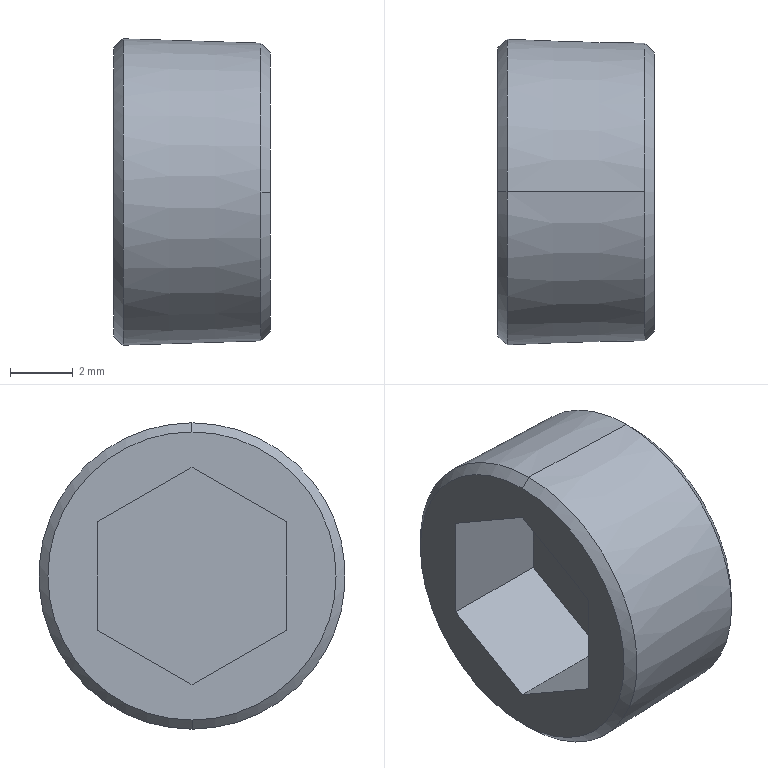Part | STEP file | 1 solid | 15 faces | box 5 x 9.772 x 9.772 mm | volume 252.752 mm3 | plane 9 | cone 6
STEP:
#1=CARTESIAN_POINT('',(0.,0.,0.));
#2=DIRECTION('',(0.,0.,1.));
#3=DIRECTION('',(1.,0.,0.));
#4=AXIS2_PLACEMENT_3D('',#1,#2,#3);
#5=CARTESIAN_POINT('',(5.,4.439,0.));
#6=VERTEX_POINT('',#5);
#7=CARTESIAN_POINT('',(5.,-4.439,0.));
#8=VERTEX_POINT('',#7);
#9=CARTESIAN_POINT('',(5.,0.,0.));
#10=DIRECTION('',(1.,0.,0.));
#11=DIRECTION('',(0.,-1.,0.));
#12=AXIS2_PLACEMENT_3D('',#9,#10,#11);
#13=CIRCLE('',#12,4.439);
#14=CARTESIAN_POINT('',(5.,0.,0.));
#15=DIRECTION('',(-1.,0.,0.));
#16=DIRECTION('',(0.,-1.,0.));
#17=AXIS2_PLACEMENT_3D('',#14,#15,#16);
#18=CONICAL_SURFACE('',#17,4.439,0.801);
#19=CARTESIAN_POINT('',(6.283,0.));
#20=DIRECTION('',(-1.,0.));
#21=VECTOR('',#20,1.);
#22=LINE('',#19,#21);
#23=(GEOMETRIC_REPRESENTATION_CONTEXT(2)PARAMETRIC_REPRESENTATION_CONTEXT()REPRESENTATION_CONTEXT('',''));
#24=DEFINITIONAL_REPRESENTATION('',(#22),#23);
#25=PCURVE('',#18,#24);
#26=CARTESIAN_POINT('',(5.,-4.492,-4.492));
#27=DIRECTION('',(-1.,0.,0.));
#28=DIRECTION('',(0.,0.,1.));
#29=AXIS2_PLACEMENT_3D('',#26,#27,#28);
#30=PLANE('',#29);
#31=CARTESIAN_POINT('',(4.492,0.05327));
#32=CARTESIAN_POINT('',(-3.196,0.05327));
#33=CARTESIAN_POINT('',(0.648,6.712));
#34=CARTESIAN_POINT('',(4.492,13.371));
#35=CARTESIAN_POINT('',(8.337,6.712));
#36=CARTESIAN_POINT('',(12.181,0.05327));
#37=CARTESIAN_POINT('',(4.492,0.05327));
#38=(BOUNDED_CURVE()B_SPLINE_CURVE(2,(#31,#32,#33,#34,#35,#36,#37),.UNSPECIFIED.,.T.,.F.)B_SPLINE_CURVE_WITH_KNOTS((1,2,2,2,2,1),(-2.094,0.,2.094,4.189,6.283,8.378),.UNSPECIFIED.)CURVE()GEOMETRIC_REPRESENTATION_ITEM()RATIONAL_B_SPLINE_CURVE((1.,0.5,1.,0.5,1.,0.5,1.))REPRESENTATION_ITEM(''));
#39=(GEOMETRIC_REPRESENTATION_CONTEXT(2)PARAMETRIC_REPRESENTATION_CONTEXT()REPRESENTATION_CONTEXT('',''));
#40=DEFINITIONAL_REPRESENTATION('',(#38),#39);
#41=PCURVE('',#30,#40);
#42=SURFACE_CURVE('',#13,(#25,#41),.PCURVE_S1.);
#43=EDGE_CURVE('',#6,#8,#42,.T.);
#44=ORIENTED_EDGE('',*,*,#43,.F.);
#45=CARTESIAN_POINT('',(4.7,4.748,0.));
#46=VERTEX_POINT('',#45);
#47=CARTESIAN_POINT('',(5.,4.439,0.));
#48=DIRECTION('',(-0.696,0.7181,0.));
#49=VECTOR('',#48,1.);
#50=LINE('',#47,#49);
#51=CARTESIAN_POINT('',(3.142,0.));
#52=DIRECTION('',(0.,1.));
#53=VECTOR('',#52,1.);
#54=LINE('',#51,#53);
#55=(GEOMETRIC_REPRESENTATION_CONTEXT(2)PARAMETRIC_REPRESENTATION_CONTEXT()REPRESENTATION_CONTEXT('',''));
#56=DEFINITIONAL_REPRESENTATION('',(#54),#55);
#57=PCURVE('',#18,#56);
#58=CARTESIAN_POINT('',(5.,0.,0.));
#59=DIRECTION('',(-1.,0.,0.));
#60=DIRECTION('',(0.,-1.,0.));
#61=AXIS2_PLACEMENT_3D('',#58,#59,#60);
#62=CONICAL_SURFACE('',#61,4.439,0.801);
#63=CARTESIAN_POINT('',(3.142,0.));
#64=DIRECTION('',(0.,1.));
#65=VECTOR('',#64,1.);
#66=LINE('',#63,#65);
#67=(GEOMETRIC_REPRESENTATION_CONTEXT(2)PARAMETRIC_REPRESENTATION_CONTEXT()REPRESENTATION_CONTEXT('',''));
#68=DEFINITIONAL_REPRESENTATION('',(#66),#67);
#69=PCURVE('',#62,#68);
#70=SURFACE_CURVE('',#50,(#57,#69),.PCURVE_S1.);
#71=EDGE_CURVE('',#6,#46,#70,.T.);
#72=ORIENTED_EDGE('',*,*,#71,.T.);
#73=CARTESIAN_POINT('',(4.7,0.,4.748));
#74=VERTEX_POINT('',#73);
#75=CARTESIAN_POINT('',(4.7,0.,0.));
#76=DIRECTION('',(-1.,0.,0.));
#77=DIRECTION('',(0.,0.,1.));
#78=AXIS2_PLACEMENT_3D('',#75,#76,#77);
#79=CIRCLE('',#78,4.748);
#80=CARTESIAN_POINT('',(1.571,0.2999));
#81=DIRECTION('',(1.,0.));
#82=VECTOR('',#81,1.);
#83=LINE('',#80,#82);
#84=(GEOMETRIC_REPRESENTATION_CONTEXT(2)PARAMETRIC_REPRESENTATION_CONTEXT()REPRESENTATION_CONTEXT('',''));
#85=DEFINITIONAL_REPRESENTATION('',(#83),#84);
#86=PCURVE('',#18,#85);
#87=CARTESIAN_POINT('',(4.7,0.,0.));
#88=DIRECTION('',(-1.,0.,0.));
#89=DIRECTION('',(0.,0.,1.));
#90=AXIS2_PLACEMENT_3D('',#87,#88,#89);
#91=CONICAL_SURFACE('',#90,4.748,0.03121);
#92=CARTESIAN_POINT('',(0.,0.));
#93=DIRECTION('',(1.,0.));
#94=VECTOR('',#93,1.);
#95=LINE('',#92,#94);
#96=(GEOMETRIC_REPRESENTATION_CONTEXT(2)PARAMETRIC_REPRESENTATION_CONTEXT()REPRESENTATION_CONTEXT('',''));
#97=DEFINITIONAL_REPRESENTATION('',(#95),#96);
#98=PCURVE('',#91,#97);
#99=SURFACE_CURVE('',#79,(#86,#98),.PCURVE_S1.);
#100=EDGE_CURVE('',#74,#46,#99,.T.);
#101=ORIENTED_EDGE('',*,*,#100,.F.);
#102=CARTESIAN_POINT('',(4.7,-4.748,0.));
#103=VERTEX_POINT('',#102);
#104=CARTESIAN_POINT('',(4.7,0.,0.));
#105=DIRECTION('',(-1.,0.,0.));
#106=DIRECTION('',(0.,0.,1.));
#107=AXIS2_PLACEMENT_3D('',#104,#105,#106);
#108=CIRCLE('',#107,4.748);
#109=CARTESIAN_POINT('',(-4.712,0.2999));
#110=DIRECTION('',(1.,0.));
#111=VECTOR('',#110,1.);
#112=LINE('',#109,#111);
#113=(GEOMETRIC_REPRESENTATION_CONTEXT(2)PARAMETRIC_REPRESENTATION_CONTEXT()REPRESENTATION_CONTEXT('',''));
#114=DEFINITIONAL_REPRESENTATION('',(#112),#113);
#115=PCURVE('',#18,#114);
#116=CARTESIAN_POINT('',(4.7,0.,0.));
#117=DIRECTION('',(-1.,0.,0.));
#118=DIRECTION('',(0.,0.,1.));
#119=AXIS2_PLACEMENT_3D('',#116,#117,#118);
#120=CONICAL_SURFACE('',#119,4.748,0.03121);
#121=CARTESIAN_POINT('',(0.,0.));
#122=DIRECTION('',(1.,0.));
#123=VECTOR('',#122,1.);
#124=LINE('',#121,#123);
#125=(GEOMETRIC_REPRESENTATION_CONTEXT(2)PARAMETRIC_REPRESENTATION_CONTEXT()REPRESENTATION_CONTEXT('',''));
#126=DEFINITIONAL_REPRESENTATION('',(#124),#125);
#127=PCURVE('',#120,#126);
#128=SURFACE_CURVE('',#108,(#115,#127),.PCURVE_S1.);
#129=EDGE_CURVE('',#103,#74,#128,.T.);
#130=ORIENTED_EDGE('',*,*,#129,.F.);
#131=CARTESIAN_POINT('',(5.,-4.439,0.));
#132=DIRECTION('',(-0.696,-0.7181,0.));
#133=VECTOR('',#132,1.);
#134=LINE('',#131,#133);
#135=CARTESIAN_POINT('',(0.,0.));
#136=DIRECTION('',(0.,1.));
#137=VECTOR('',#136,1.);
#138=LINE('',#135,#137);
#139=(GEOMETRIC_REPRESENTATION_CONTEXT(2)PARAMETRIC_REPRESENTATION_CONTEXT()REPRESENTATION_CONTEXT('',''));
#140=DEFINITIONAL_REPRESENTATION('',(#138),#139);
#141=PCURVE('',#18,#140);
#142=CARTESIAN_POINT('',(6.283,0.));
#143=DIRECTION('',(0.,1.));
#144=VECTOR('',#143,1.);
#145=LINE('',#142,#144);
#146=(GEOMETRIC_REPRESENTATION_CONTEXT(2)PARAMETRIC_REPRESENTATION_CONTEXT()REPRESENTATION_CONTEXT('',''));
#147=DEFINITIONAL_REPRESENTATION('',(#145),#146);
#148=PCURVE('',#62,#147);
#149=SURFACE_CURVE('',#134,(#141,#148),.PCURVE_S1.);
#150=EDGE_CURVE('',#8,#103,#149,.T.);
#151=ORIENTED_EDGE('',*,*,#150,.F.);
#152=EDGE_LOOP('',(#44,#72,#101,#130,#151));
#153=FACE_BOUND('',#152,.T.);
#154=ADVANCED_FACE('',(#153),#18,.T.);
#155=ORIENTED_EDGE('',*,*,#100,.T.);
#156=CARTESIAN_POINT('',(4.7,0.,-4.748));
#157=VERTEX_POINT('',#156);
#158=CARTESIAN_POINT('',(4.7,0.,0.));
#159=DIRECTION('',(-1.,0.,0.));
#160=DIRECTION('',(0.,0.,1.));
#161=AXIS2_PLACEMENT_3D('',#158,#159,#160);
#162=CIRCLE('',#161,4.748);
#163=CARTESIAN_POINT('',(0.,0.));
#164=DIRECTION('',(1.,0.));
#165=VECTOR('',#164,1.);
#166=LINE('',#163,#165);
#167=(GEOMETRIC_REPRESENTATION_CONTEXT(2)PARAMETRIC_REPRESENTATION_CONTEXT()REPRESENTATION_CONTEXT('',''));
#168=DEFINITIONAL_REPRESENTATION('',(#166),#167);
#169=PCURVE('',#91,#168);
#170=CARTESIAN_POINT('',(1.571,0.2999));
#171=DIRECTION('',(1.,0.));
#172=VECTOR('',#171,1.);
#173=LINE('',#170,#172);
#174=(GEOMETRIC_REPRESENTATION_CONTEXT(2)PARAMETRIC_REPRESENTATION_CONTEXT()REPRESENTATION_CONTEXT('',''));
#175=DEFINITIONAL_REPRESENTATION('',(#173),#174);
#176=PCURVE('',#62,#175);
#177=SURFACE_CURVE('',#162,(#169,#176),.PCURVE_S1.);
#178=EDGE_CURVE('',#46,#157,#177,.T.);
#179=ORIENTED_EDGE('',*,*,#178,.T.);
#180=CARTESIAN_POINT('',(0.2999,0.,-4.886));
#181=VERTEX_POINT('',#180);
#182=CARTESIAN_POINT('',(4.7,0.,-4.748));
#183=DIRECTION('',(-0.9995,0.,-0.0312));
#184=VECTOR('',#183,1.);
#185=LINE('',#182,#184);
#186=CARTESIAN_POINT('',(3.142,0.));
#187=DIRECTION('',(0.,1.));
#188=VECTOR('',#187,1.);
#189=LINE('',#186,#188);
#190=(GEOMETRIC_REPRESENTATION_CONTEXT(2)PARAMETRIC_REPRESENTATION_CONTEXT()REPRESENTATION_CONTEXT('',''));
#191=DEFINITIONAL_REPRESENTATION('',(#189),#190);
#192=PCURVE('',#91,#191);
#193=CARTESIAN_POINT('',(3.142,0.));
#194=DIRECTION('',(0.,1.));
#195=VECTOR('',#194,1.);
#196=LINE('',#193,#195);
#197=(GEOMETRIC_REPRESENTATION_CONTEXT(2)PARAMETRIC_REPRESENTATION_CONTEXT()REPRESENTATION_CONTEXT('',''));
#198=DEFINITIONAL_REPRESENTATION('',(#196),#197);
#199=PCURVE('',#120,#198);
#200=SURFACE_CURVE('',#185,(#192,#199),.PCURVE_S1.);
#201=EDGE_CURVE('',#157,#181,#200,.T.);
#202=ORIENTED_EDGE('',*,*,#201,.T.);
#203=CARTESIAN_POINT('',(0.2999,0.,4.886));
#204=VERTEX_POINT('',#203);
#205=CARTESIAN_POINT('',(0.2999,0.,0.));
#206=DIRECTION('',(-1.,0.,0.));
#207=DIRECTION('',(0.,0.,1.));
#208=AXIS2_PLACEMENT_3D('',#205,#206,#207);
#209=CIRCLE('',#208,4.886);
#210=CARTESIAN_POINT('',(0.,4.4));
#211=DIRECTION('',(1.,0.));
#212=VECTOR('',#211,1.);
#213=LINE('',#210,#212);
#214=(GEOMETRIC_REPRESENTATION_CONTEXT(2)PARAMETRIC_REPRESENTATION_CONTEXT()REPRESENTATION_CONTEXT('',''));
#215=DEFINITIONAL_REPRESENTATION('',(#213),#214);
#216=PCURVE('',#91,#215);
#217=CARTESIAN_POINT('',(0.,0.,0.));
#218=DIRECTION('',(1.,0.,0.));
#219=DIRECTION('',(0.,0.,-1.));
#220=AXIS2_PLACEMENT_3D('',#217,#218,#219);
#221=CONICAL_SURFACE('',#220,4.595,0.7698);
#222=CARTESIAN_POINT('',(3.142,0.2999));
#223=DIRECTION('',(-1.,0.));
#224=VECTOR('',#223,1.);
#225=LINE('',#222,#224);
#226=(GEOMETRIC_REPRESENTATION_CONTEXT(2)PARAMETRIC_REPRESENTATION_CONTEXT()REPRESENTATION_CONTEXT('',''));
#227=DEFINITIONAL_REPRESENTATION('',(#225),#226);
#228=PCURVE('',#221,#227);
#229=SURFACE_CURVE('',#209,(#216,#228),.PCURVE_S1.);
#230=EDGE_CURVE('',#204,#181,#229,.T.);
#231=ORIENTED_EDGE('',*,*,#230,.F.);
#232=CARTESIAN_POINT('',(4.7,0.,4.748));
#233=DIRECTION('',(-0.9995,0.,0.0312));
#234=VECTOR('',#233,1.);
#235=LINE('',#232,#234);
#236=CARTESIAN_POINT('',(0.,0.));
#237=DIRECTION('',(0.,1.));
#238=VECTOR('',#237,1.);
#239=LINE('',#236,#238);
#240=(GEOMETRIC_REPRESENTATION_CONTEXT(2)PARAMETRIC_REPRESENTATION_CONTEXT()REPRESENTATION_CONTEXT('',''));
#241=DEFINITIONAL_REPRESENTATION('',(#239),#240);
#242=PCURVE('',#91,#241);
#243=CARTESIAN_POINT('',(6.283,0.));
#244=DIRECTION('',(0.,1.));
#245=VECTOR('',#244,1.);
#246=LINE('',#243,#245);
#247=(GEOMETRIC_REPRESENTATION_CONTEXT(2)PARAMETRIC_REPRESENTATION_CONTEXT()REPRESENTATION_CONTEXT('',''));
#248=DEFINITIONAL_REPRESENTATION('',(#246),#247);
#249=PCURVE('',#120,#248);
#250=SURFACE_CURVE('',#235,(#242,#249),.PCURVE_S1.);
#251=EDGE_CURVE('',#74,#204,#250,.T.);
#252=ORIENTED_EDGE('',*,*,#251,.F.);
#253=EDGE_LOOP('',(#155,#179,#202,#231,#252));
#254=FACE_BOUND('',#253,.T.);
#255=ADVANCED_FACE('',(#254),#91,.T.);
#256=CARTESIAN_POINT('',(0.,0.,4.595));
#257=VERTEX_POINT('',#256);
#258=CARTESIAN_POINT('',(0.,0.,-4.595));
#259=VERTEX_POINT('',#258);
#260=CARTESIAN_POINT('',(0.,0.,0.));
#261=DIRECTION('',(-1.,0.,0.));
#262=DIRECTION('',(0.,0.,-1.));
#263=AXIS2_PLACEMENT_3D('',#260,#261,#262);
#264=CIRCLE('',#263,4.595);
#265=CARTESIAN_POINT('',(6.283,0.));
#266=DIRECTION('',(-1.,0.));
#267=VECTOR('',#266,1.);
#268=LINE('',#265,#267);
#269=(GEOMETRIC_REPRESENTATION_CONTEXT(2)PARAMETRIC_REPRESENTATION_CONTEXT()REPRESENTATION_CONTEXT('',''));
#270=DEFINITIONAL_REPRESENTATION('',(#268),#269);
#271=PCURVE('',#221,#270);
#272=CARTESIAN_POINT('',(0.,-4.65,4.65));
#273=DIRECTION('',(1.,0.,0.));
#274=DIRECTION('',(0.,0.,-1.));
#275=AXIS2_PLACEMENT_3D('',#272,#273,#274);
#276=PLANE('',#275);
#277=CARTESIAN_POINT('',(9.246,4.65));
#278=CARTESIAN_POINT('',(9.246,-3.309));
#279=CARTESIAN_POINT('',(2.353,0.6708));
#280=CARTESIAN_POINT('',(-4.54,4.65));
#281=CARTESIAN_POINT('',(2.353,8.63));
#282=CARTESIAN_POINT('',(9.246,12.61));
#283=CARTESIAN_POINT('',(9.246,4.65));
#284=(BOUNDED_CURVE()B_SPLINE_CURVE(2,(#277,#278,#279,#280,#281,#282,#283),.UNSPECIFIED.,.T.,.F.)B_SPLINE_CURVE_WITH_KNOTS((1,2,2,2,2,1),(-2.094,0.,2.094,4.189,6.283,8.378),.UNSPECIFIED.)CURVE()GEOMETRIC_REPRESENTATION_ITEM()RATIONAL_B_SPLINE_CURVE((1.,0.5,1.,0.5,1.,0.5,1.))REPRESENTATION_ITEM(''));
#285=(GEOMETRIC_REPRESENTATION_CONTEXT(2)PARAMETRIC_REPRESENTATION_CONTEXT()REPRESENTATION_CONTEXT('',''));
#286=DEFINITIONAL_REPRESENTATION('',(#284),#285);
#287=PCURVE('',#276,#286);
#288=SURFACE_CURVE('',#264,(#271,#287),.PCURVE_S1.);
#289=EDGE_CURVE('',#257,#259,#288,.T.);
#290=ORIENTED_EDGE('',*,*,#289,.F.);
#291=CARTESIAN_POINT('',(0.,0.,4.595));
#292=DIRECTION('',(0.7181,0.,0.696));
#293=VECTOR('',#292,1.);
#294=LINE('',#291,#293);
#295=CARTESIAN_POINT('',(3.142,0.));
#296=DIRECTION('',(0.,1.));
#297=VECTOR('',#296,1.);
#298=LINE('',#295,#297);
#299=(GEOMETRIC_REPRESENTATION_CONTEXT(2)PARAMETRIC_REPRESENTATION_CONTEXT()REPRESENTATION_CONTEXT('',''));
#300=DEFINITIONAL_REPRESENTATION('',(#298),#299);
#301=PCURVE('',#221,#300);
#302=CARTESIAN_POINT('',(0.,0.,0.));
#303=DIRECTION('',(1.,0.,0.));
#304=DIRECTION('',(0.,0.,-1.));
#305=AXIS2_PLACEMENT_3D('',#302,#303,#304);
#306=CONICAL_SURFACE('',#305,4.595,0.7698);
#307=CARTESIAN_POINT('',(3.142,0.));
#308=DIRECTION('',(0.,1.));
#309=VECTOR('',#308,1.);
#310=LINE('',#307,#309);
#311=(GEOMETRIC_REPRESENTATION_CONTEXT(2)PARAMETRIC_REPRESENTATION_CONTEXT()REPRESENTATION_CONTEXT('',''));
#312=DEFINITIONAL_REPRESENTATION('',(#310),#311);
#313=PCURVE('',#306,#312);
#314=SURFACE_CURVE('',#294,(#301,#313),.PCURVE_S1.);
#315=EDGE_CURVE('',#257,#204,#314,.T.);
#316=ORIENTED_EDGE('',*,*,#315,.T.);
#317=ORIENTED_EDGE('',*,*,#230,.T.);
#318=CARTESIAN_POINT('',(0.,0.,-4.595));
#319=DIRECTION('',(0.7181,0.,-0.696));
#320=VECTOR('',#319,1.);
#321=LINE('',#318,#320);
#322=CARTESIAN_POINT('',(0.,0.));
#323=DIRECTION('',(0.,1.));
#324=VECTOR('',#323,1.);
#325=LINE('',#322,#324);
#326=(GEOMETRIC_REPRESENTATION_CONTEXT(2)PARAMETRIC_REPRESENTATION_CONTEXT()REPRESENTATION_CONTEXT('',''));
#327=DEFINITIONAL_REPRESENTATION('',(#325),#326);
#328=PCURVE('',#221,#327);
#329=CARTESIAN_POINT('',(6.283,0.));
#330=DIRECTION('',(0.,1.));
#331=VECTOR('',#330,1.);
#332=LINE('',#329,#331);
#333=(GEOMETRIC_REPRESENTATION_CONTEXT(2)PARAMETRIC_REPRESENTATION_CONTEXT()REPRESENTATION_CONTEXT('',''));
#334=DEFINITIONAL_REPRESENTATION('',(#332),#333);
#335=PCURVE('',#306,#334);
#336=SURFACE_CURVE('',#321,(#328,#335),.PCURVE_S1.);
#337=EDGE_CURVE('',#259,#181,#336,.T.);
#338=ORIENTED_EDGE('',*,*,#337,.F.);
#339=EDGE_LOOP('',(#290,#316,#317,#338));
#340=FACE_BOUND('',#339,.T.);
#341=ADVANCED_FACE('',(#340),#221,.T.);
#342=ORIENTED_EDGE('',*,*,#71,.F.);
#343=CARTESIAN_POINT('',(5.,0.,0.));
#344=DIRECTION('',(1.,0.,0.));
#345=DIRECTION('',(0.,-1.,0.));
#346=AXIS2_PLACEMENT_3D('',#343,#344,#345);
#347=CIRCLE('',#346,4.439);
#348=CARTESIAN_POINT('',(6.283,0.));
#349=DIRECTION('',(-1.,0.));
#350=VECTOR('',#349,1.);
#351=LINE('',#348,#350);
#352=(GEOMETRIC_REPRESENTATION_CONTEXT(2)PARAMETRIC_REPRESENTATION_CONTEXT()REPRESENTATION_CONTEXT('',''));
#353=DEFINITIONAL_REPRESENTATION('',(#351),#352);
#354=PCURVE('',#62,#353);
#355=CARTESIAN_POINT('',(4.492,0.05327));
#356=CARTESIAN_POINT('',(-3.196,0.05327));
#357=CARTESIAN_POINT('',(0.648,6.712));
#358=CARTESIAN_POINT('',(4.492,13.371));
#359=CARTESIAN_POINT('',(8.337,6.712));
#360=CARTESIAN_POINT('',(12.181,0.05327));
#361=CARTESIAN_POINT('',(4.492,0.05327));
#362=(BOUNDED_CURVE()B_SPLINE_CURVE(2,(#355,#356,#357,#358,#359,#360,#361),.UNSPECIFIED.,.T.,.F.)B_SPLINE_CURVE_WITH_KNOTS((1,2,2,2,2,1),(-2.094,0.,2.094,4.189,6.283,8.378),.UNSPECIFIED.)CURVE()GEOMETRIC_REPRESENTATION_ITEM()RATIONAL_B_SPLINE_CURVE((1.,0.5,1.,0.5,1.,0.5,1.))REPRESENTATION_ITEM(''));
#363=(GEOMETRIC_REPRESENTATION_CONTEXT(2)PARAMETRIC_REPRESENTATION_CONTEXT()REPRESENTATION_CONTEXT('',''));
#364=DEFINITIONAL_REPRESENTATION('',(#362),#363);
#365=PCURVE('',#30,#364);
#366=SURFACE_CURVE('',#347,(#354,#365),.PCURVE_S1.);
#367=EDGE_CURVE('',#8,#6,#366,.T.);
#368=ORIENTED_EDGE('',*,*,#367,.F.);
#369=ORIENTED_EDGE('',*,*,#150,.T.);
#370=CARTESIAN_POINT('',(4.7,0.,0.));
#371=DIRECTION('',(-1.,0.,0.));
#372=DIRECTION('',(0.,0.,1.));
#373=AXIS2_PLACEMENT_3D('',#370,#371,#372);
#374=CIRCLE('',#373,4.748);
#375=CARTESIAN_POINT('',(1.571,0.2999));
#376=DIRECTION('',(1.,0.));
#377=VECTOR('',#376,1.);
#378=LINE('',#375,#377);
#379=(GEOMETRIC_REPRESENTATION_CONTEXT(2)PARAMETRIC_REPRESENTATION_CONTEXT()REPRESENTATION_CONTEXT('',''));
#380=DEFINITIONAL_REPRESENTATION('',(#378),#379);
#381=PCURVE('',#62,#380);
#382=CARTESIAN_POINT('',(0.,0.));
#383=DIRECTION('',(1.,0.));
#384=VECTOR('',#383,1.);
#385=LINE('',#382,#384);
#386=(GEOMETRIC_REPRESENTATION_CONTEXT(2)PARAMETRIC_REPRESENTATION_CONTEXT()REPRESENTATION_CONTEXT('',''));
#387=DEFINITIONAL_REPRESENTATION('',(#385),#386);
#388=PCURVE('',#120,#387);
#389=SURFACE_CURVE('',#374,(#381,#388),.PCURVE_S1.);
#390=EDGE_CURVE('',#157,#103,#389,.T.);
#391=ORIENTED_EDGE('',*,*,#390,.F.);
#392=ORIENTED_EDGE('',*,*,#178,.F.);
#393=EDGE_LOOP('',(#342,#368,#369,#391,#392));
#394=FACE_BOUND('',#393,.T.);
#395=ADVANCED_FACE('',(#394),#62,.T.);
#396=ORIENTED_EDGE('',*,*,#367,.T.);
#397=ORIENTED_EDGE('',*,*,#43,.T.);
#398=EDGE_LOOP('',(#396,#397));
#399=FACE_BOUND('',#398,.T.);
#400=ADVANCED_FACE('',(#399),#30,.F.);
#401=ORIENTED_EDGE('',*,*,#201,.F.);
#402=ORIENTED_EDGE('',*,*,#390,.T.);
#403=ORIENTED_EDGE('',*,*,#129,.T.);
#404=ORIENTED_EDGE('',*,*,#251,.T.);
#405=CARTESIAN_POINT('',(0.2999,0.,0.));
#406=DIRECTION('',(-1.,0.,0.));
#407=DIRECTION('',(0.,0.,1.));
#408=AXIS2_PLACEMENT_3D('',#405,#406,#407);
#409=CIRCLE('',#408,4.886);
#410=CARTESIAN_POINT('',(0.,4.4));
#411=DIRECTION('',(1.,0.));
#412=VECTOR('',#411,1.);
#413=LINE('',#410,#412);
#414=(GEOMETRIC_REPRESENTATION_CONTEXT(2)PARAMETRIC_REPRESENTATION_CONTEXT()REPRESENTATION_CONTEXT('',''));
#415=DEFINITIONAL_REPRESENTATION('',(#413),#414);
#416=PCURVE('',#120,#415);
#417=CARTESIAN_POINT('',(9.425,0.2999));
#418=DIRECTION('',(-1.,0.));
#419=VECTOR('',#418,1.);
#420=LINE('',#417,#419);
#421=(GEOMETRIC_REPRESENTATION_CONTEXT(2)PARAMETRIC_REPRESENTATION_CONTEXT()REPRESENTATION_CONTEXT('',''));
#422=DEFINITIONAL_REPRESENTATION('',(#420),#421);
#423=PCURVE('',#306,#422);
#424=SURFACE_CURVE('',#409,(#416,#423),.PCURVE_S1.);
#425=EDGE_CURVE('',#181,#204,#424,.T.);
#426=ORIENTED_EDGE('',*,*,#425,.F.);
#427=EDGE_LOOP('',(#401,#402,#403,#404,#426));
#428=FACE_BOUND('',#427,.T.);
#429=ADVANCED_FACE('',(#428),#120,.T.);
#430=ORIENTED_EDGE('',*,*,#315,.F.);
#431=CARTESIAN_POINT('',(0.,0.,0.));
#432=DIRECTION('',(-1.,0.,0.));
#433=DIRECTION('',(0.,0.,-1.));
#434=AXIS2_PLACEMENT_3D('',#431,#432,#433);
#435=CIRCLE('',#434,4.595);
#436=CARTESIAN_POINT('',(6.283,0.));
#437=DIRECTION('',(-1.,0.));
#438=VECTOR('',#437,1.);
#439=LINE('',#436,#438);
#440=(GEOMETRIC_REPRESENTATION_CONTEXT(2)PARAMETRIC_REPRESENTATION_CONTEXT()REPRESENTATION_CONTEXT('',''));
#441=DEFINITIONAL_REPRESENTATION('',(#439),#440);
#442=PCURVE('',#306,#441);
#443=CARTESIAN_POINT('',(9.246,4.65));
#444=CARTESIAN_POINT('',(9.246,-3.309));
#445=CARTESIAN_POINT('',(2.353,0.6708));
#446=CARTESIAN_POINT('',(-4.54,4.65));
#447=CARTESIAN_POINT('',(2.353,8.63));
#448=CARTESIAN_POINT('',(9.246,12.61));
#449=CARTESIAN_POINT('',(9.246,4.65));
#450=(BOUNDED_CURVE()B_SPLINE_CURVE(2,(#443,#444,#445,#446,#447,#448,#449),.UNSPECIFIED.,.T.,.F.)B_SPLINE_CURVE_WITH_KNOTS((1,2,2,2,2,1),(-2.094,0.,2.094,4.189,6.283,8.378),.UNSPECIFIED.)CURVE()GEOMETRIC_REPRESENTATION_ITEM()RATIONAL_B_SPLINE_CURVE((1.,0.5,1.,0.5,1.,0.5,1.))REPRESENTATION_ITEM(''));
#451=(GEOMETRIC_REPRESENTATION_CONTEXT(2)PARAMETRIC_REPRESENTATION_CONTEXT()REPRESENTATION_CONTEXT('',''));
#452=DEFINITIONAL_REPRESENTATION('',(#450),#451);
#453=PCURVE('',#276,#452);
#454=SURFACE_CURVE('',#435,(#442,#453),.PCURVE_S1.);
#455=EDGE_CURVE('',#259,#257,#454,.T.);
#456=ORIENTED_EDGE('',*,*,#455,.F.);
#457=ORIENTED_EDGE('',*,*,#337,.T.);
#458=ORIENTED_EDGE('',*,*,#425,.T.);
#459=EDGE_LOOP('',(#430,#456,#457,#458));
#460=FACE_BOUND('',#459,.T.);
#461=ADVANCED_FACE('',(#460),#306,.T.);
#462=CARTESIAN_POINT('',(0.,0.,-3.464));
#463=VERTEX_POINT('',#462);
#464=CARTESIAN_POINT('',(0.,-3.,-1.732));
#465=VERTEX_POINT('',#464);
#466=CARTESIAN_POINT('',(0.,-3.,-1.732));
#467=DIRECTION('',(0.,-0.866,0.5));
#468=VECTOR('',#467,1.);
#469=LINE('',#466,#468);
#470=CARTESIAN_POINT('',(6.382,1.65));
#471=DIRECTION('',(-0.5,-0.866));
#472=VECTOR('',#471,1.);
#473=LINE('',#470,#472);
#474=(GEOMETRIC_REPRESENTATION_CONTEXT(2)PARAMETRIC_REPRESENTATION_CONTEXT()REPRESENTATION_CONTEXT('',''));
#475=DEFINITIONAL_REPRESENTATION('',(#473),#474);
#476=PCURVE('',#276,#475);
#477=CARTESIAN_POINT('',(0.,-3.,-1.732));
#478=DIRECTION('',(0.,-0.5,-0.866));
#479=DIRECTION('',(0.,0.866,-0.5));
#480=AXIS2_PLACEMENT_3D('',#477,#478,#479);
#481=PLANE('',#480);
#482=CARTESIAN_POINT('',(0.,0.));
#483=DIRECTION('',(-1.,0.));
#484=VECTOR('',#483,1.);
#485=LINE('',#482,#484);
#486=(GEOMETRIC_REPRESENTATION_CONTEXT(2)PARAMETRIC_REPRESENTATION_CONTEXT()REPRESENTATION_CONTEXT('',''));
#487=DEFINITIONAL_REPRESENTATION('',(#485),#486);
#488=PCURVE('',#481,#487);
#489=SURFACE_CURVE('',#469,(#476,#488),.PCURVE_S1.);
#490=EDGE_CURVE('',#463,#465,#489,.T.);
#491=ORIENTED_EDGE('',*,*,#490,.F.);
#492=CARTESIAN_POINT('',(0.,3.,-1.732));
#493=VERTEX_POINT('',#492);
#494=CARTESIAN_POINT('',(0.,0.,-3.464));
#495=DIRECTION('',(0.,-0.866,-0.5));
#496=VECTOR('',#495,1.);
#497=LINE('',#494,#496);
#498=CARTESIAN_POINT('',(8.114,4.65));
#499=DIRECTION('',(0.5,-0.866));
#500=VECTOR('',#499,1.);
#501=LINE('',#498,#500);
#502=(GEOMETRIC_REPRESENTATION_CONTEXT(2)PARAMETRIC_REPRESENTATION_CONTEXT()REPRESENTATION_CONTEXT('',''));
#503=DEFINITIONAL_REPRESENTATION('',(#501),#502);
#504=PCURVE('',#276,#503);
#505=CARTESIAN_POINT('',(0.,0.,-3.464));
#506=DIRECTION('',(0.,0.5,-0.866));
#507=DIRECTION('',(0.,0.866,0.5));
#508=AXIS2_PLACEMENT_3D('',#505,#506,#507);
#509=PLANE('',#508);
#510=CARTESIAN_POINT('',(0.,0.));
#511=DIRECTION('',(-1.,0.));
#512=VECTOR('',#511,1.);
#513=LINE('',#510,#512);
#514=(GEOMETRIC_REPRESENTATION_CONTEXT(2)PARAMETRIC_REPRESENTATION_CONTEXT()REPRESENTATION_CONTEXT('',''));
#515=DEFINITIONAL_REPRESENTATION('',(#513),#514);
#516=PCURVE('',#509,#515);
#517=SURFACE_CURVE('',#497,(#504,#516),.PCURVE_S1.);
#518=EDGE_CURVE('',#493,#463,#517,.T.);
#519=ORIENTED_EDGE('',*,*,#518,.F.);
#520=CARTESIAN_POINT('',(0.,3.,1.732));
#521=VERTEX_POINT('',#520);
#522=CARTESIAN_POINT('',(0.,3.,0.));
#523=DIRECTION('',(0.,0.,-1.));
#524=VECTOR('',#523,1.);
#525=LINE('',#522,#524);
#526=CARTESIAN_POINT('',(4.65,7.65));
#527=DIRECTION('',(1.,0.));
#528=VECTOR('',#527,1.);
#529=LINE('',#526,#528);
#530=(GEOMETRIC_REPRESENTATION_CONTEXT(2)PARAMETRIC_REPRESENTATION_CONTEXT()REPRESENTATION_CONTEXT('',''));
#531=DEFINITIONAL_REPRESENTATION('',(#529),#530);
#532=PCURVE('',#276,#531);
#533=CARTESIAN_POINT('',(0.,3.,-1.732));
#534=DIRECTION('',(0.,1.,0.));
#535=DIRECTION('',(0.,0.,1.));
#536=AXIS2_PLACEMENT_3D('',#533,#534,#535);
#537=PLANE('',#536);
#538=CARTESIAN_POINT('',(1.732,0.));
#539=DIRECTION('',(-1.,0.));
#540=VECTOR('',#539,1.);
#541=LINE('',#538,#540);
#542=(GEOMETRIC_REPRESENTATION_CONTEXT(2)PARAMETRIC_REPRESENTATION_CONTEXT()REPRESENTATION_CONTEXT('',''));
#543=DEFINITIONAL_REPRESENTATION('',(#541),#542);
#544=PCURVE('',#537,#543);
#545=SURFACE_CURVE('',#525,(#532,#544),.PCURVE_S1.);
#546=EDGE_CURVE('',#521,#493,#545,.T.);
#547=ORIENTED_EDGE('',*,*,#546,.F.);
#548=CARTESIAN_POINT('',(0.,0.,3.464));
#549=VERTEX_POINT('',#548);
#550=CARTESIAN_POINT('',(0.,3.,1.732));
#551=DIRECTION('',(0.,0.866,-0.5));
#552=VECTOR('',#551,1.);
#553=LINE('',#550,#552);
#554=CARTESIAN_POINT('',(2.918,7.65));
#555=DIRECTION('',(0.5,0.866));
#556=VECTOR('',#555,1.);
#557=LINE('',#554,#556);
#558=(GEOMETRIC_REPRESENTATION_CONTEXT(2)PARAMETRIC_REPRESENTATION_CONTEXT()REPRESENTATION_CONTEXT('',''));
#559=DEFINITIONAL_REPRESENTATION('',(#557),#558);
#560=PCURVE('',#276,#559);
#561=CARTESIAN_POINT('',(0.,3.,1.732));
#562=DIRECTION('',(0.,0.5,0.866));
#563=DIRECTION('',(0.,-0.866,0.5));
#564=AXIS2_PLACEMENT_3D('',#561,#562,#563);
#565=PLANE('',#564);
#566=CARTESIAN_POINT('',(0.,0.));
#567=DIRECTION('',(-1.,0.));
#568=VECTOR('',#567,1.);
#569=LINE('',#566,#568);
#570=(GEOMETRIC_REPRESENTATION_CONTEXT(2)PARAMETRIC_REPRESENTATION_CONTEXT()REPRESENTATION_CONTEXT('',''));
#571=DEFINITIONAL_REPRESENTATION('',(#569),#570);
#572=PCURVE('',#565,#571);
#573=SURFACE_CURVE('',#553,(#560,#572),.PCURVE_S1.);
#574=EDGE_CURVE('',#549,#521,#573,.T.);
#575=ORIENTED_EDGE('',*,*,#574,.F.);
#576=CARTESIAN_POINT('',(0.,-3.,1.732));
#577=VERTEX_POINT('',#576);
#578=CARTESIAN_POINT('',(0.,0.,3.464));
#579=DIRECTION('',(0.,0.866,0.5));
#580=VECTOR('',#579,1.);
#581=LINE('',#578,#580);
#582=CARTESIAN_POINT('',(1.186,4.65));
#583=DIRECTION('',(-0.5,0.866));
#584=VECTOR('',#583,1.);
#585=LINE('',#582,#584);
#586=(GEOMETRIC_REPRESENTATION_CONTEXT(2)PARAMETRIC_REPRESENTATION_CONTEXT()REPRESENTATION_CONTEXT('',''));
#587=DEFINITIONAL_REPRESENTATION('',(#585),#586);
#588=PCURVE('',#276,#587);
#589=CARTESIAN_POINT('',(0.,0.,3.464));
#590=DIRECTION('',(0.,-0.5,0.866));
#591=DIRECTION('',(0.,-0.866,-0.5));
#592=AXIS2_PLACEMENT_3D('',#589,#590,#591);
#593=PLANE('',#592);
#594=CARTESIAN_POINT('',(0.,0.));
#595=DIRECTION('',(-1.,0.));
#596=VECTOR('',#595,1.);
#597=LINE('',#594,#596);
#598=(GEOMETRIC_REPRESENTATION_CONTEXT(2)PARAMETRIC_REPRESENTATION_CONTEXT()REPRESENTATION_CONTEXT('',''));
#599=DEFINITIONAL_REPRESENTATION('',(#597),#598);
#600=PCURVE('',#593,#599);
#601=SURFACE_CURVE('',#581,(#588,#600),.PCURVE_S1.);
#602=EDGE_CURVE('',#577,#549,#601,.T.);
#603=ORIENTED_EDGE('',*,*,#602,.F.);
#604=CARTESIAN_POINT('',(0.,-3.,0.));
#605=DIRECTION('',(0.,0.,1.));
#606=VECTOR('',#605,1.);
#607=LINE('',#604,#606);
#608=CARTESIAN_POINT('',(4.65,1.65));
#609=DIRECTION('',(-1.,0.));
#610=VECTOR('',#609,1.);
#611=LINE('',#608,#610);
#612=(GEOMETRIC_REPRESENTATION_CONTEXT(2)PARAMETRIC_REPRESENTATION_CONTEXT()REPRESENTATION_CONTEXT('',''));
#613=DEFINITIONAL_REPRESENTATION('',(#611),#612);
#614=PCURVE('',#276,#613);
#615=CARTESIAN_POINT('',(0.,-3.,1.732));
#616=DIRECTION('',(0.,-1.,0.));
#617=DIRECTION('',(0.,0.,-1.));
#618=AXIS2_PLACEMENT_3D('',#615,#616,#617);
#619=PLANE('',#618);
#620=CARTESIAN_POINT('',(1.732,0.));
#621=DIRECTION('',(-1.,0.));
#622=VECTOR('',#621,1.);
#623=LINE('',#620,#622);
#624=(GEOMETRIC_REPRESENTATION_CONTEXT(2)PARAMETRIC_REPRESENTATION_CONTEXT()REPRESENTATION_CONTEXT('',''));
#625=DEFINITIONAL_REPRESENTATION('',(#623),#624);
#626=PCURVE('',#619,#625);
#627=SURFACE_CURVE('',#607,(#614,#626),.PCURVE_S1.);
#628=EDGE_CURVE('',#465,#577,#627,.T.);
#629=ORIENTED_EDGE('',*,*,#628,.F.);
#630=EDGE_LOOP('',(#491,#519,#547,#575,#603,#629));
#631=FACE_BOUND('',#630,.T.);
#632=ORIENTED_EDGE('',*,*,#455,.T.);
#633=ORIENTED_EDGE('',*,*,#289,.T.);
#634=EDGE_LOOP('',(#632,#633));
#635=FACE_BOUND('',#634,.T.);
#636=ADVANCED_FACE('',(#631,#635),#276,.F.);
#637=CARTESIAN_POINT('',(3.5,-3.,1.732));
#638=VERTEX_POINT('',#637);
#639=CARTESIAN_POINT('',(1.75,-3.,1.732));
#640=DIRECTION('',(-1.,0.,0.));
#641=VECTOR('',#640,1.);
#642=LINE('',#639,#641);
#643=CARTESIAN_POINT('',(0.,1.75));
#644=DIRECTION('',(0.,-1.));
#645=VECTOR('',#644,1.);
#646=LINE('',#643,#645);
#647=(GEOMETRIC_REPRESENTATION_CONTEXT(2)PARAMETRIC_REPRESENTATION_CONTEXT()REPRESENTATION_CONTEXT('',''));
#648=DEFINITIONAL_REPRESENTATION('',(#646),#647);
#649=PCURVE('',#619,#648);
#650=CARTESIAN_POINT('',(3.464,1.75));
#651=DIRECTION('',(0.,-1.));
#652=VECTOR('',#651,1.);
#653=LINE('',#650,#652);
#654=(GEOMETRIC_REPRESENTATION_CONTEXT(2)PARAMETRIC_REPRESENTATION_CONTEXT()REPRESENTATION_CONTEXT('',''));
#655=DEFINITIONAL_REPRESENTATION('',(#653),#654);
#656=PCURVE('',#593,#655);
#657=SURFACE_CURVE('',#642,(#649,#656),.PCURVE_S1.);
#658=EDGE_CURVE('',#638,#577,#657,.T.);
#659=ORIENTED_EDGE('',*,*,#658,.F.);
#660=CARTESIAN_POINT('',(3.5,-3.,-1.732));
#661=VERTEX_POINT('',#660);
#662=CARTESIAN_POINT('',(3.5,-3.,0.));
#663=DIRECTION('',(0.,0.,1.));
#664=VECTOR('',#663,1.);
#665=LINE('',#662,#664);
#666=CARTESIAN_POINT('',(1.732,3.5));
#667=DIRECTION('',(-1.,0.));
#668=VECTOR('',#667,1.);
#669=LINE('',#666,#668);
#670=(GEOMETRIC_REPRESENTATION_CONTEXT(2)PARAMETRIC_REPRESENTATION_CONTEXT()REPRESENTATION_CONTEXT('',''));
#671=DEFINITIONAL_REPRESENTATION('',(#669),#670);
#672=PCURVE('',#619,#671);
#673=CARTESIAN_POINT('',(3.5,-3.,-3.464));
#674=DIRECTION('',(-1.,0.,0.));
#675=DIRECTION('',(0.,0.,1.));
#676=AXIS2_PLACEMENT_3D('',#673,#674,#675);
#677=PLANE('',#676);
#678=CARTESIAN_POINT('',(3.464,0.));
#679=DIRECTION('',(1.,0.));
#680=VECTOR('',#679,1.);
#681=LINE('',#678,#680);
#682=(GEOMETRIC_REPRESENTATION_CONTEXT(2)PARAMETRIC_REPRESENTATION_CONTEXT()REPRESENTATION_CONTEXT('',''));
#683=DEFINITIONAL_REPRESENTATION('',(#681),#682);
#684=PCURVE('',#677,#683);
#685=SURFACE_CURVE('',#665,(#672,#684),.PCURVE_S1.);
#686=EDGE_CURVE('',#661,#638,#685,.T.);
#687=ORIENTED_EDGE('',*,*,#686,.F.);
#688=CARTESIAN_POINT('',(1.75,-3.,-1.732));
#689=DIRECTION('',(1.,0.,0.));
#690=VECTOR('',#689,1.);
#691=LINE('',#688,#690);
#692=CARTESIAN_POINT('',(3.464,1.75));
#693=DIRECTION('',(0.,1.));
#694=VECTOR('',#693,1.);
#695=LINE('',#692,#694);
#696=(GEOMETRIC_REPRESENTATION_CONTEXT(2)PARAMETRIC_REPRESENTATION_CONTEXT()REPRESENTATION_CONTEXT('',''));
#697=DEFINITIONAL_REPRESENTATION('',(#695),#696);
#698=PCURVE('',#619,#697);
#699=CARTESIAN_POINT('',(0.,1.75));
#700=DIRECTION('',(0.,1.));
#701=VECTOR('',#700,1.);
#702=LINE('',#699,#701);
#703=(GEOMETRIC_REPRESENTATION_CONTEXT(2)PARAMETRIC_REPRESENTATION_CONTEXT()REPRESENTATION_CONTEXT('',''));
#704=DEFINITIONAL_REPRESENTATION('',(#702),#703);
#705=PCURVE('',#481,#704);
#706=SURFACE_CURVE('',#691,(#698,#705),.PCURVE_S1.);
#707=EDGE_CURVE('',#465,#661,#706,.T.);
#708=ORIENTED_EDGE('',*,*,#707,.F.);
#709=ORIENTED_EDGE('',*,*,#628,.T.);
#710=EDGE_LOOP('',(#659,#687,#708,#709));
#711=FACE_BOUND('',#710,.T.);
#712=ADVANCED_FACE('',(#711),#619,.F.);
#713=ORIENTED_EDGE('',*,*,#707,.T.);
#714=CARTESIAN_POINT('',(3.5,-0.000000001,-3.464));
#715=VERTEX_POINT('',#714);
#716=CARTESIAN_POINT('',(3.5,-1.5,-2.598));
#717=DIRECTION('',(0.,-0.866,0.5));
#718=VECTOR('',#717,1.);
#719=LINE('',#716,#718);
#720=CARTESIAN_POINT('',(1.732,3.5));
#721=DIRECTION('',(-1.,0.));
#722=VECTOR('',#721,1.);
#723=LINE('',#720,#722);
#724=(GEOMETRIC_REPRESENTATION_CONTEXT(2)PARAMETRIC_REPRESENTATION_CONTEXT()REPRESENTATION_CONTEXT('',''));
#725=DEFINITIONAL_REPRESENTATION('',(#723),#724);
#726=PCURVE('',#481,#725);
#727=CARTESIAN_POINT('',(0.866,1.5));
#728=DIRECTION('',(0.5,-0.866));
#729=VECTOR('',#728,1.);
#730=LINE('',#727,#729);
#731=(GEOMETRIC_REPRESENTATION_CONTEXT(2)PARAMETRIC_REPRESENTATION_CONTEXT()REPRESENTATION_CONTEXT('',''));
#732=DEFINITIONAL_REPRESENTATION('',(#730),#731);
#733=PCURVE('',#677,#732);
#734=SURFACE_CURVE('',#719,(#726,#733),.PCURVE_S1.);
#735=EDGE_CURVE('',#715,#661,#734,.T.);
#736=ORIENTED_EDGE('',*,*,#735,.F.);
#737=CARTESIAN_POINT('',(1.75,0.,-3.464));
#738=DIRECTION('',(1.,0.,0.));
#739=VECTOR('',#738,1.);
#740=LINE('',#737,#739);
#741=CARTESIAN_POINT('',(3.464,1.75));
#742=DIRECTION('',(0.,1.));
#743=VECTOR('',#742,1.);
#744=LINE('',#741,#743);
#745=(GEOMETRIC_REPRESENTATION_CONTEXT(2)PARAMETRIC_REPRESENTATION_CONTEXT()REPRESENTATION_CONTEXT('',''));
#746=DEFINITIONAL_REPRESENTATION('',(#744),#745);
#747=PCURVE('',#481,#746);
#748=CARTESIAN_POINT('',(0.,1.75));
#749=DIRECTION('',(0.,1.));
#750=VECTOR('',#749,1.);
#751=LINE('',#748,#750);
#752=(GEOMETRIC_REPRESENTATION_CONTEXT(2)PARAMETRIC_REPRESENTATION_CONTEXT()REPRESENTATION_CONTEXT('',''));
#753=DEFINITIONAL_REPRESENTATION('',(#751),#752);
#754=PCURVE('',#509,#753);
#755=SURFACE_CURVE('',#740,(#747,#754),.PCURVE_S1.);
#756=EDGE_CURVE('',#463,#715,#755,.T.);
#757=ORIENTED_EDGE('',*,*,#756,.F.);
#758=ORIENTED_EDGE('',*,*,#490,.T.);
#759=EDGE_LOOP('',(#713,#736,#757,#758));
#760=FACE_BOUND('',#759,.T.);
#761=ADVANCED_FACE('',(#760),#481,.F.);
#762=ORIENTED_EDGE('',*,*,#756,.T.);
#763=CARTESIAN_POINT('',(3.5,3.,-1.732));
#764=VERTEX_POINT('',#763);
#765=CARTESIAN_POINT('',(3.5,1.5,-2.598));
#766=DIRECTION('',(0.,-0.866,-0.5));
#767=VECTOR('',#766,1.);
#768=LINE('',#765,#767);
#769=CARTESIAN_POINT('',(1.732,3.5));
#770=DIRECTION('',(-1.,0.));
#771=VECTOR('',#770,1.);
#772=LINE('',#769,#771);
#773=(GEOMETRIC_REPRESENTATION_CONTEXT(2)PARAMETRIC_REPRESENTATION_CONTEXT()REPRESENTATION_CONTEXT('',''));
#774=DEFINITIONAL_REPRESENTATION('',(#772),#773);
#775=PCURVE('',#509,#774);
#776=CARTESIAN_POINT('',(0.866,4.5));
#777=DIRECTION('',(-0.5,-0.866));
#778=VECTOR('',#777,1.);
#779=LINE('',#776,#778);
#780=(GEOMETRIC_REPRESENTATION_CONTEXT(2)PARAMETRIC_REPRESENTATION_CONTEXT()REPRESENTATION_CONTEXT('',''));
#781=DEFINITIONAL_REPRESENTATION('',(#779),#780);
#782=PCURVE('',#677,#781);
#783=SURFACE_CURVE('',#768,(#775,#782),.PCURVE_S1.);
#784=EDGE_CURVE('',#764,#715,#783,.T.);
#785=ORIENTED_EDGE('',*,*,#784,.F.);
#786=CARTESIAN_POINT('',(1.75,3.,-1.732));
#787=DIRECTION('',(1.,0.,0.));
#788=VECTOR('',#787,1.);
#789=LINE('',#786,#788);
#790=CARTESIAN_POINT('',(3.464,1.75));
#791=DIRECTION('',(0.,1.));
#792=VECTOR('',#791,1.);
#793=LINE('',#790,#792);
#794=(GEOMETRIC_REPRESENTATION_CONTEXT(2)PARAMETRIC_REPRESENTATION_CONTEXT()REPRESENTATION_CONTEXT('',''));
#795=DEFINITIONAL_REPRESENTATION('',(#793),#794);
#796=PCURVE('',#509,#795);
#797=CARTESIAN_POINT('',(0.,1.75));
#798=DIRECTION('',(0.,1.));
#799=VECTOR('',#798,1.);
#800=LINE('',#797,#799);
#801=(GEOMETRIC_REPRESENTATION_CONTEXT(2)PARAMETRIC_REPRESENTATION_CONTEXT()REPRESENTATION_CONTEXT('',''));
#802=DEFINITIONAL_REPRESENTATION('',(#800),#801);
#803=PCURVE('',#537,#802);
#804=SURFACE_CURVE('',#789,(#796,#803),.PCURVE_S1.);
#805=EDGE_CURVE('',#493,#764,#804,.T.);
#806=ORIENTED_EDGE('',*,*,#805,.F.);
#807=ORIENTED_EDGE('',*,*,#518,.T.);
#808=EDGE_LOOP('',(#762,#785,#806,#807));
#809=FACE_BOUND('',#808,.T.);
#810=ADVANCED_FACE('',(#809),#509,.F.);
#811=ORIENTED_EDGE('',*,*,#805,.T.);
#812=CARTESIAN_POINT('',(3.5,3.,1.732));
#813=VERTEX_POINT('',#812);
#814=CARTESIAN_POINT('',(3.5,3.,0.));
#815=DIRECTION('',(0.,0.,-1.));
#816=VECTOR('',#815,1.);
#817=LINE('',#814,#816);
#818=CARTESIAN_POINT('',(1.732,3.5));
#819=DIRECTION('',(-1.,0.));
#820=VECTOR('',#819,1.);
#821=LINE('',#818,#820);
#822=(GEOMETRIC_REPRESENTATION_CONTEXT(2)PARAMETRIC_REPRESENTATION_CONTEXT()REPRESENTATION_CONTEXT('',''));
#823=DEFINITIONAL_REPRESENTATION('',(#821),#822);
#824=PCURVE('',#537,#823);
#825=CARTESIAN_POINT('',(3.464,6.));
#826=DIRECTION('',(-1.,0.));
#827=VECTOR('',#826,1.);
#828=LINE('',#825,#827);
#829=(GEOMETRIC_REPRESENTATION_CONTEXT(2)PARAMETRIC_REPRESENTATION_CONTEXT()REPRESENTATION_CONTEXT('',''));
#830=DEFINITIONAL_REPRESENTATION('',(#828),#829);
#831=PCURVE('',#677,#830);
#832=SURFACE_CURVE('',#817,(#824,#831),.PCURVE_S1.);
#833=EDGE_CURVE('',#813,#764,#832,.T.);
#834=ORIENTED_EDGE('',*,*,#833,.F.);
#835=CARTESIAN_POINT('',(1.75,3.,1.732));
#836=DIRECTION('',(1.,0.,0.));
#837=VECTOR('',#836,1.);
#838=LINE('',#835,#837);
#839=CARTESIAN_POINT('',(3.464,1.75));
#840=DIRECTION('',(0.,1.));
#841=VECTOR('',#840,1.);
#842=LINE('',#839,#841);
#843=(GEOMETRIC_REPRESENTATION_CONTEXT(2)PARAMETRIC_REPRESENTATION_CONTEXT()REPRESENTATION_CONTEXT('',''));
#844=DEFINITIONAL_REPRESENTATION('',(#842),#843);
#845=PCURVE('',#537,#844);
#846=CARTESIAN_POINT('',(0.,1.75));
#847=DIRECTION('',(0.,1.));
#848=VECTOR('',#847,1.);
#849=LINE('',#846,#848);
#850=(GEOMETRIC_REPRESENTATION_CONTEXT(2)PARAMETRIC_REPRESENTATION_CONTEXT()REPRESENTATION_CONTEXT('',''));
#851=DEFINITIONAL_REPRESENTATION('',(#849),#850);
#852=PCURVE('',#565,#851);
#853=SURFACE_CURVE('',#838,(#845,#852),.PCURVE_S1.);
#854=EDGE_CURVE('',#521,#813,#853,.T.);
#855=ORIENTED_EDGE('',*,*,#854,.F.);
#856=ORIENTED_EDGE('',*,*,#546,.T.);
#857=EDGE_LOOP('',(#811,#834,#855,#856));
#858=FACE_BOUND('',#857,.T.);
#859=ADVANCED_FACE('',(#858),#537,.F.);
#860=ORIENTED_EDGE('',*,*,#854,.T.);
#861=CARTESIAN_POINT('',(3.5,-0.000000001,3.464));
#862=VERTEX_POINT('',#861);
#863=CARTESIAN_POINT('',(3.5,1.5,2.598));
#864=DIRECTION('',(0.,0.866,-0.5));
#865=VECTOR('',#864,1.);
#866=LINE('',#863,#865);
#867=CARTESIAN_POINT('',(1.732,3.5));
#868=DIRECTION('',(-1.,0.));
#869=VECTOR('',#868,1.);
#870=LINE('',#867,#869);
#871=(GEOMETRIC_REPRESENTATION_CONTEXT(2)PARAMETRIC_REPRESENTATION_CONTEXT()REPRESENTATION_CONTEXT('',''));
#872=DEFINITIONAL_REPRESENTATION('',(#870),#871);
#873=PCURVE('',#565,#872);
#874=CARTESIAN_POINT('',(6.062,4.5));
#875=DIRECTION('',(-0.5,0.866));
#876=VECTOR('',#875,1.);
#877=LINE('',#874,#876);
#878=(GEOMETRIC_REPRESENTATION_CONTEXT(2)PARAMETRIC_REPRESENTATION_CONTEXT()REPRESENTATION_CONTEXT('',''));
#879=DEFINITIONAL_REPRESENTATION('',(#877),#878);
#880=PCURVE('',#677,#879);
#881=SURFACE_CURVE('',#866,(#873,#880),.PCURVE_S1.);
#882=EDGE_CURVE('',#862,#813,#881,.T.);
#883=ORIENTED_EDGE('',*,*,#882,.F.);
#884=CARTESIAN_POINT('',(1.75,0.,3.464));
#885=DIRECTION('',(1.,0.,0.));
#886=VECTOR('',#885,1.);
#887=LINE('',#884,#886);
#888=CARTESIAN_POINT('',(3.464,1.75));
#889=DIRECTION('',(0.,1.));
#890=VECTOR('',#889,1.);
#891=LINE('',#888,#890);
#892=(GEOMETRIC_REPRESENTATION_CONTEXT(2)PARAMETRIC_REPRESENTATION_CONTEXT()REPRESENTATION_CONTEXT('',''));
#893=DEFINITIONAL_REPRESENTATION('',(#891),#892);
#894=PCURVE('',#565,#893);
#895=CARTESIAN_POINT('',(0.,1.75));
#896=DIRECTION('',(0.,1.));
#897=VECTOR('',#896,1.);
#898=LINE('',#895,#897);
#899=(GEOMETRIC_REPRESENTATION_CONTEXT(2)PARAMETRIC_REPRESENTATION_CONTEXT()REPRESENTATION_CONTEXT('',''));
#900=DEFINITIONAL_REPRESENTATION('',(#898),#899);
#901=PCURVE('',#593,#900);
#902=SURFACE_CURVE('',#887,(#894,#901),.PCURVE_S1.);
#903=EDGE_CURVE('',#549,#862,#902,.T.);
#904=ORIENTED_EDGE('',*,*,#903,.F.);
#905=ORIENTED_EDGE('',*,*,#574,.T.);
#906=EDGE_LOOP('',(#860,#883,#904,#905));
#907=FACE_BOUND('',#906,.T.);
#908=ADVANCED_FACE('',(#907),#565,.F.);
#909=ORIENTED_EDGE('',*,*,#903,.T.);
#910=CARTESIAN_POINT('',(3.5,-1.5,2.598));
#911=DIRECTION('',(0.,0.866,0.5));
#912=VECTOR('',#911,1.);
#913=LINE('',#910,#912);
#914=CARTESIAN_POINT('',(1.732,3.5));
#915=DIRECTION('',(-1.,0.));
#916=VECTOR('',#915,1.);
#917=LINE('',#914,#916);
#918=(GEOMETRIC_REPRESENTATION_CONTEXT(2)PARAMETRIC_REPRESENTATION_CONTEXT()REPRESENTATION_CONTEXT('',''));
#919=DEFINITIONAL_REPRESENTATION('',(#917),#918);
#920=PCURVE('',#593,#919);
#921=CARTESIAN_POINT('',(6.062,1.5));
#922=DIRECTION('',(0.5,0.866));
#923=VECTOR('',#922,1.);
#924=LINE('',#921,#923);
#925=(GEOMETRIC_REPRESENTATION_CONTEXT(2)PARAMETRIC_REPRESENTATION_CONTEXT()REPRESENTATION_CONTEXT('',''));
#926=DEFINITIONAL_REPRESENTATION('',(#924),#925);
#927=PCURVE('',#677,#926);
#928=SURFACE_CURVE('',#913,(#920,#927),.PCURVE_S1.);
#929=EDGE_CURVE('',#638,#862,#928,.T.);
#930=ORIENTED_EDGE('',*,*,#929,.F.);
#931=ORIENTED_EDGE('',*,*,#658,.T.);
#932=ORIENTED_EDGE('',*,*,#602,.T.);
#933=EDGE_LOOP('',(#909,#930,#931,#932));
#934=FACE_BOUND('',#933,.T.);
#935=ADVANCED_FACE('',(#934),#593,.F.);
#936=ORIENTED_EDGE('',*,*,#833,.T.);
#937=ORIENTED_EDGE('',*,*,#784,.T.);
#938=ORIENTED_EDGE('',*,*,#735,.T.);
#939=ORIENTED_EDGE('',*,*,#686,.T.);
#940=ORIENTED_EDGE('',*,*,#929,.T.);
#941=ORIENTED_EDGE('',*,*,#882,.T.);
#942=EDGE_LOOP('',(#936,#937,#938,#939,#940,#941));
#943=FACE_BOUND('',#942,.T.);
#944=ADVANCED_FACE('',(#943),#677,.T.);
#945=CLOSED_SHELL('',(#154,#255,#341,#395,#400,#429,#461,#636,#712,#761,#810,#859,#908,#935,#944));
#946=MANIFOLD_SOLID_BREP('',#945);
#947=(LENGTH_UNIT()NAMED_UNIT(*)SI_UNIT(.MILLI.,.METRE.));
#948=UNCERTAINTY_MEASURE_WITH_UNIT(LENGTH_MEASURE(0.0000001),#947,'','');
#949=(NAMED_UNIT(*)PLANE_ANGLE_UNIT()SI_UNIT($,.RADIAN.));
#950=(NAMED_UNIT(*)SI_UNIT($,.STERADIAN.)SOLID_ANGLE_UNIT());
#951=(GEOMETRIC_REPRESENTATION_CONTEXT(3)GLOBAL_UNCERTAINTY_ASSIGNED_CONTEXT((#948))GLOBAL_UNIT_ASSIGNED_CONTEXT((#947,#949,#950))REPRESENTATION_CONTEXT('',''));
#952=ADVANCED_BREP_SHAPE_REPRESENTATION('',(#4,#946),#951);